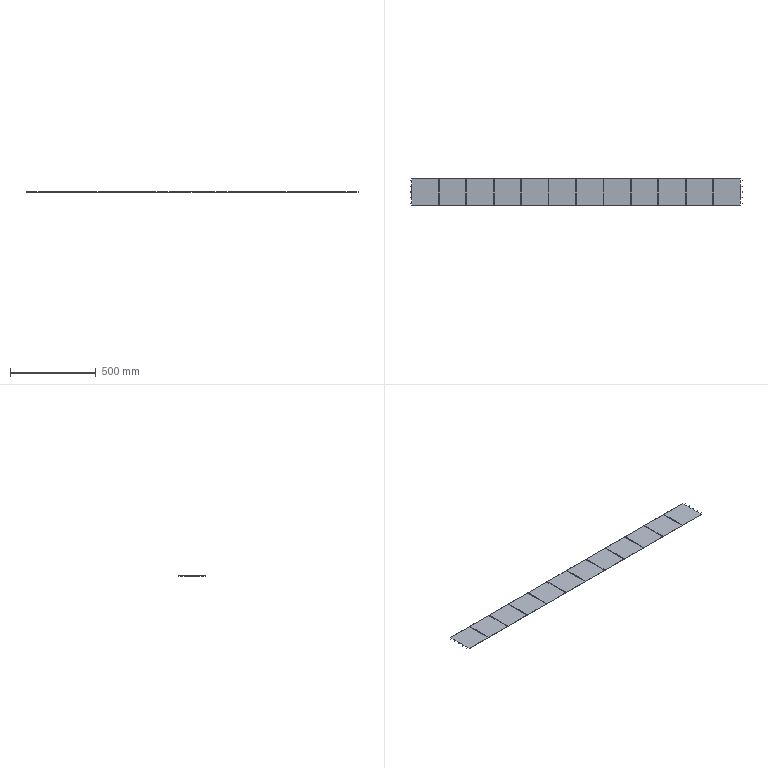Part | SolidWorks | features ICE 2, Extrusion 1, MirrorPattern 1 | 1 solid | 90 faces | box 1936 x 156 x 1.1 mm | volume 328319 mm3 | plane 90